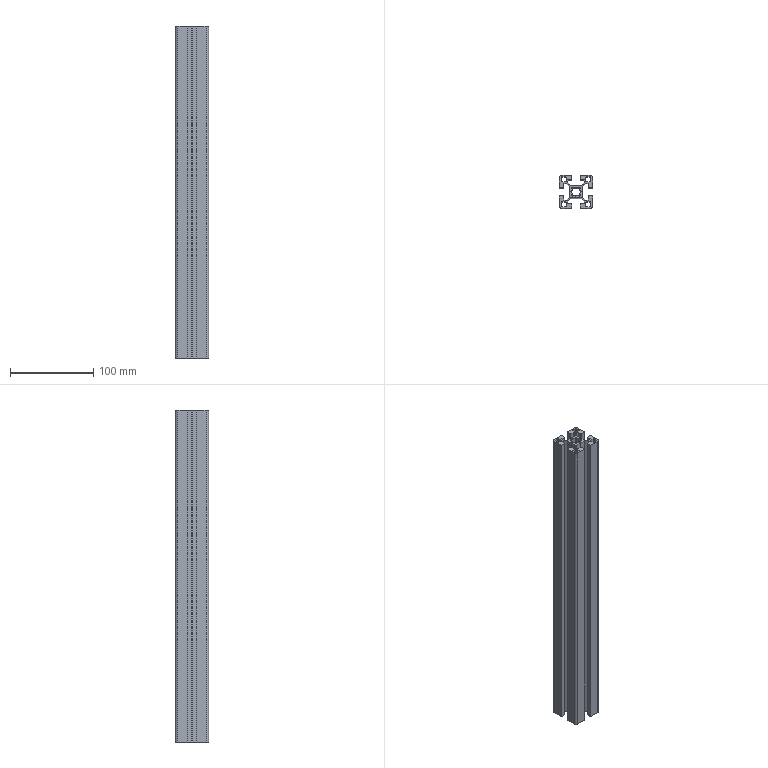Part | STEP file | 1.6米HFS8-4040-400 | 1 solid | 111 faces | box 40 x 40 x 400 mm | volume 248820 mm3 | plane 74 | cylinder 37 | commonest cylinder face diameters 2 x28 10.5 x5 6 x4